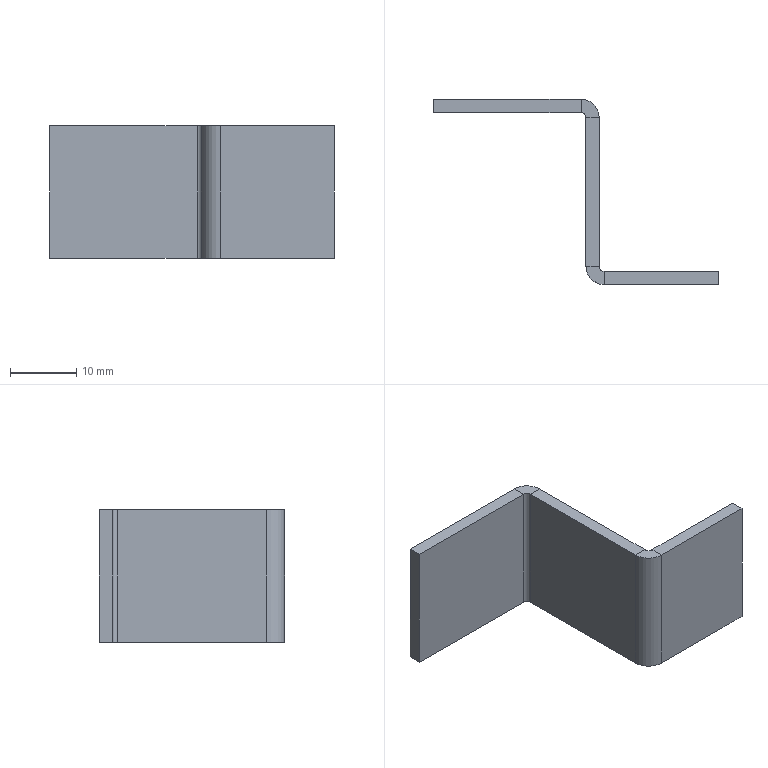Part | SolidWorks | features FlatPattern 1, SMBaseFlange 1, SheetMetal 1 | 1 solid | 22 faces | box 43 x 28 x 20 mm | volume 2700 mm3 | plane 18 | cylinder 4 | commonest cylinder face diameters 1.473 x2 5.473 x2
STEP:
#1=CARTESIAN_POINT('',(25.,-2.737,10.));
#2=VERTEX_POINT('',#1);
#3=CARTESIAN_POINT('',(23.,-2.737,10.));
#4=VERTEX_POINT('',#3);
#5=CARTESIAN_POINT('',(25.,-2.737,10.));
#6=DIRECTION('',(-1.,0.,0.));
#7=VECTOR('',#6,1000.);
#8=LINE('',#5,#7);
#9=EDGE_CURVE('',#2,#4,#8,.T.);
#10=ORIENTED_EDGE('',*,*,#9,.F.);
#11=CARTESIAN_POINT('',(22.263,0.,10.));
#12=VERTEX_POINT('',#11);
#13=CARTESIAN_POINT('',(22.263,-2.737,10.));
#14=DIRECTION('',(0.,0.,-1.));
#15=DIRECTION('',(1.,0.,0.));
#16=AXIS2_PLACEMENT_3D('',#13,#14,#15);
#17=CIRCLE('',#16,2.737);
#18=EDGE_CURVE('',#12,#2,#17,.T.);
#19=ORIENTED_EDGE('',*,*,#18,.F.);
#20=CARTESIAN_POINT('',(22.263,-2.,10.));
#21=VERTEX_POINT('',#20);
#22=CARTESIAN_POINT('',(22.263,-2.,10.));
#23=DIRECTION('',(0.,1.,0.));
#24=VECTOR('',#23,1000.);
#25=LINE('',#22,#24);
#26=EDGE_CURVE('',#21,#12,#25,.T.);
#27=ORIENTED_EDGE('',*,*,#26,.F.);
#28=CARTESIAN_POINT('',(22.263,-2.737,10.));
#29=DIRECTION('',(0.,0.,-1.));
#30=DIRECTION('',(1.,0.,0.));
#31=AXIS2_PLACEMENT_3D('',#28,#29,#30);
#32=CIRCLE('',#31,0.7366);
#33=EDGE_CURVE('',#21,#4,#32,.T.);
#34=ORIENTED_EDGE('',*,*,#33,.T.);
#35=EDGE_LOOP('',(#10,#19,#27,#34));
#36=FACE_OUTER_BOUND('',#35,.T.);
#37=CARTESIAN_POINT('',(25.,-2.737,10.));
#38=DIRECTION('',(0.,0.,1.));
#39=DIRECTION('',(1.,0.,0.));
#40=AXIS2_PLACEMENT_3D('',#37,#38,#39);
#41=PLANE('',#40);
#42=ADVANCED_FACE('',(#36),#41,.T.);
#43=CARTESIAN_POINT('',(25.,-25.263,10.));
#44=VERTEX_POINT('',#43);
#45=CARTESIAN_POINT('',(25.,0.,10.));
#46=DIRECTION('',(0.,-1.,0.));
#47=VECTOR('',#46,1000.);
#48=LINE('',#45,#47);
#49=EDGE_CURVE('',#2,#44,#48,.T.);
#50=ORIENTED_EDGE('',*,*,#49,.F.);
#51=ORIENTED_EDGE('',*,*,#9,.T.);
#52=CARTESIAN_POINT('',(23.,-25.263,10.));
#53=VERTEX_POINT('',#52);
#54=CARTESIAN_POINT('',(23.,0.,10.));
#55=DIRECTION('',(0.,-1.,0.));
#56=VECTOR('',#55,1000.);
#57=LINE('',#54,#56);
#58=EDGE_CURVE('',#4,#53,#57,.T.);
#59=ORIENTED_EDGE('',*,*,#58,.T.);
#60=CARTESIAN_POINT('',(23.,-25.263,10.));
#61=DIRECTION('',(1.,0.,0.));
#62=VECTOR('',#61,1000.);
#63=LINE('',#60,#62);
#64=EDGE_CURVE('',#53,#44,#63,.T.);
#65=ORIENTED_EDGE('',*,*,#64,.T.);
#66=EDGE_LOOP('',(#50,#51,#59,#65));
#67=FACE_OUTER_BOUND('',#66,.T.);
#68=CARTESIAN_POINT('',(22.263,-2.,10.));
#69=DIRECTION('',(0.,0.,1.));
#70=DIRECTION('',(1.,0.,0.));
#71=AXIS2_PLACEMENT_3D('',#68,#69,#70);
#72=PLANE('',#71);
#73=ADVANCED_FACE('',(#67),#72,.T.);
#74=CARTESIAN_POINT('',(22.263,0.,-10.));
#75=VERTEX_POINT('',#74);
#76=CARTESIAN_POINT('',(22.263,-2.,-10.));
#77=VERTEX_POINT('',#76);
#78=CARTESIAN_POINT('',(22.263,0.,-10.));
#79=DIRECTION('',(0.,-1.,0.));
#80=VECTOR('',#79,1000.);
#81=LINE('',#78,#80);
#82=EDGE_CURVE('',#75,#77,#81,.T.);
#83=ORIENTED_EDGE('',*,*,#82,.F.);
#84=CARTESIAN_POINT('',(25.,-2.737,-10.));
#85=VERTEX_POINT('',#84);
#86=CARTESIAN_POINT('',(22.263,-2.737,-10.));
#87=DIRECTION('',(0.,0.,-1.));
#88=DIRECTION('',(1.,0.,0.));
#89=AXIS2_PLACEMENT_3D('',#86,#87,#88);
#90=CIRCLE('',#89,2.737);
#91=EDGE_CURVE('',#75,#85,#90,.T.);
#92=ORIENTED_EDGE('',*,*,#91,.T.);
#93=CARTESIAN_POINT('',(23.,-2.737,-10.));
#94=VERTEX_POINT('',#93);
#95=CARTESIAN_POINT('',(23.,-2.737,-10.));
#96=DIRECTION('',(1.,0.,0.));
#97=VECTOR('',#96,1000.);
#98=LINE('',#95,#97);
#99=EDGE_CURVE('',#94,#85,#98,.T.);
#100=ORIENTED_EDGE('',*,*,#99,.F.);
#101=CARTESIAN_POINT('',(22.263,-2.737,-10.));
#102=DIRECTION('',(0.,0.,-1.));
#103=DIRECTION('',(1.,0.,0.));
#104=AXIS2_PLACEMENT_3D('',#101,#102,#103);
#105=CIRCLE('',#104,0.7366);
#106=EDGE_CURVE('',#77,#94,#105,.T.);
#107=ORIENTED_EDGE('',*,*,#106,.F.);
#108=EDGE_LOOP('',(#83,#92,#100,#107));
#109=FACE_OUTER_BOUND('',#108,.T.);
#110=CARTESIAN_POINT('',(22.263,0.,-10.));
#111=DIRECTION('',(0.,0.,-1.));
#112=DIRECTION('',(-1.,0.,0.));
#113=AXIS2_PLACEMENT_3D('',#110,#111,#112);
#114=PLANE('',#113);
#115=ADVANCED_FACE('',(#109),#114,.T.);
#116=CARTESIAN_POINT('',(0.,0.,-10.));
#117=VERTEX_POINT('',#116);
#118=CARTESIAN_POINT('',(0.,0.,-10.));
#119=DIRECTION('',(1.,0.,0.));
#120=VECTOR('',#119,1000.);
#121=LINE('',#118,#120);
#122=EDGE_CURVE('',#117,#75,#121,.T.);
#123=ORIENTED_EDGE('',*,*,#122,.T.);
#124=ORIENTED_EDGE('',*,*,#82,.T.);
#125=CARTESIAN_POINT('',(0.,-2.,-10.));
#126=VERTEX_POINT('',#125);
#127=CARTESIAN_POINT('',(0.,-2.,-10.));
#128=DIRECTION('',(1.,0.,0.));
#129=VECTOR('',#128,1000.);
#130=LINE('',#127,#129);
#131=EDGE_CURVE('',#126,#77,#130,.T.);
#132=ORIENTED_EDGE('',*,*,#131,.F.);
#133=CARTESIAN_POINT('',(0.,-2.,-10.));
#134=DIRECTION('',(0.,1.,0.));
#135=VECTOR('',#134,1000.);
#136=LINE('',#133,#135);
#137=EDGE_CURVE('',#126,#117,#136,.T.);
#138=ORIENTED_EDGE('',*,*,#137,.T.);
#139=EDGE_LOOP('',(#123,#124,#132,#138));
#140=FACE_OUTER_BOUND('',#139,.T.);
#141=CARTESIAN_POINT('',(23.,-2.737,-10.));
#142=DIRECTION('',(0.,0.,-1.));
#143=DIRECTION('',(-1.,0.,0.));
#144=AXIS2_PLACEMENT_3D('',#141,#142,#143);
#145=PLANE('',#144);
#146=ADVANCED_FACE('',(#140),#145,.T.);
#147=CARTESIAN_POINT('',(25.737,-26.,10.));
#148=VERTEX_POINT('',#147);
#149=CARTESIAN_POINT('',(25.737,-28.,10.));
#150=VERTEX_POINT('',#149);
#151=CARTESIAN_POINT('',(25.737,-26.,10.));
#152=DIRECTION('',(0.,-1.,0.));
#153=VECTOR('',#152,1000.);
#154=LINE('',#151,#153);
#155=EDGE_CURVE('',#148,#150,#154,.T.);
#156=ORIENTED_EDGE('',*,*,#155,.F.);
#157=CARTESIAN_POINT('',(25.737,-25.263,10.));
#158=DIRECTION('',(0.,0.,1.));
#159=DIRECTION('',(-1.,0.,0.));
#160=AXIS2_PLACEMENT_3D('',#157,#158,#159);
#161=CIRCLE('',#160,0.7366);
#162=EDGE_CURVE('',#44,#148,#161,.T.);
#163=ORIENTED_EDGE('',*,*,#162,.F.);
#164=ORIENTED_EDGE('',*,*,#64,.F.);
#165=CARTESIAN_POINT('',(25.737,-25.263,10.));
#166=DIRECTION('',(0.,0.,1.));
#167=DIRECTION('',(1.,0.,0.));
#168=AXIS2_PLACEMENT_3D('',#165,#166,#167);
#169=CIRCLE('',#168,2.737);
#170=EDGE_CURVE('',#53,#150,#169,.T.);
#171=ORIENTED_EDGE('',*,*,#170,.T.);
#172=EDGE_LOOP('',(#156,#163,#164,#171));
#173=FACE_OUTER_BOUND('',#172,.T.);
#174=CARTESIAN_POINT('',(25.737,-26.,10.));
#175=DIRECTION('',(0.,0.,1.));
#176=DIRECTION('',(1.,0.,0.));
#177=AXIS2_PLACEMENT_3D('',#174,#175,#176);
#178=PLANE('',#177);
#179=ADVANCED_FACE('',(#173),#178,.T.);
#180=CARTESIAN_POINT('',(43.,-26.,10.));
#181=VERTEX_POINT('',#180);
#182=CARTESIAN_POINT('',(25.,-26.,10.));
#183=DIRECTION('',(1.,0.,0.));
#184=VECTOR('',#183,1000.);
#185=LINE('',#182,#184);
#186=EDGE_CURVE('',#148,#181,#185,.T.);
#187=ORIENTED_EDGE('',*,*,#186,.F.);
#188=ORIENTED_EDGE('',*,*,#155,.T.);
#189=CARTESIAN_POINT('',(43.,-28.,10.));
#190=VERTEX_POINT('',#189);
#191=CARTESIAN_POINT('',(25.,-28.,10.));
#192=DIRECTION('',(1.,0.,0.));
#193=VECTOR('',#192,1000.);
#194=LINE('',#191,#193);
#195=EDGE_CURVE('',#150,#190,#194,.T.);
#196=ORIENTED_EDGE('',*,*,#195,.T.);
#197=CARTESIAN_POINT('',(43.,-26.,10.));
#198=DIRECTION('',(0.,-1.,0.));
#199=VECTOR('',#198,1000.);
#200=LINE('',#197,#199);
#201=EDGE_CURVE('',#181,#190,#200,.T.);
#202=ORIENTED_EDGE('',*,*,#201,.F.);
#203=EDGE_LOOP('',(#187,#188,#196,#202));
#204=FACE_OUTER_BOUND('',#203,.T.);
#205=CARTESIAN_POINT('',(23.,-25.263,10.));
#206=DIRECTION('',(0.,0.,1.));
#207=DIRECTION('',(1.,0.,0.));
#208=AXIS2_PLACEMENT_3D('',#205,#206,#207);
#209=PLANE('',#208);
#210=ADVANCED_FACE('',(#204),#209,.T.);
#211=CARTESIAN_POINT('',(25.,-25.263,-10.));
#212=VERTEX_POINT('',#211);
#213=CARTESIAN_POINT('',(23.,-25.263,-10.));
#214=VERTEX_POINT('',#213);
#215=CARTESIAN_POINT('',(25.,-25.263,-10.));
#216=DIRECTION('',(-1.,0.,0.));
#217=VECTOR('',#216,1000.);
#218=LINE('',#215,#217);
#219=EDGE_CURVE('',#212,#214,#218,.T.);
#220=ORIENTED_EDGE('',*,*,#219,.F.);
#221=CARTESIAN_POINT('',(25.737,-26.,-10.));
#222=VERTEX_POINT('',#221);
#223=CARTESIAN_POINT('',(25.737,-25.263,-10.));
#224=DIRECTION('',(0.,0.,1.));
#225=DIRECTION('',(-1.,0.,0.));
#226=AXIS2_PLACEMENT_3D('',#223,#224,#225);
#227=CIRCLE('',#226,0.7366);
#228=EDGE_CURVE('',#212,#222,#227,.T.);
#229=ORIENTED_EDGE('',*,*,#228,.T.);
#230=CARTESIAN_POINT('',(25.737,-28.,-10.));
#231=VERTEX_POINT('',#230);
#232=CARTESIAN_POINT('',(25.737,-28.,-10.));
#233=DIRECTION('',(0.,1.,0.));
#234=VECTOR('',#233,1000.);
#235=LINE('',#232,#234);
#236=EDGE_CURVE('',#231,#222,#235,.T.);
#237=ORIENTED_EDGE('',*,*,#236,.F.);
#238=CARTESIAN_POINT('',(25.737,-25.263,-10.));
#239=DIRECTION('',(0.,0.,1.));
#240=DIRECTION('',(1.,0.,0.));
#241=AXIS2_PLACEMENT_3D('',#238,#239,#240);
#242=CIRCLE('',#241,2.737);
#243=EDGE_CURVE('',#214,#231,#242,.T.);
#244=ORIENTED_EDGE('',*,*,#243,.F.);
#245=EDGE_LOOP('',(#220,#229,#237,#244));
#246=FACE_OUTER_BOUND('',#245,.T.);
#247=CARTESIAN_POINT('',(25.,-25.263,-10.));
#248=DIRECTION('',(0.,0.,-1.));
#249=DIRECTION('',(-1.,0.,0.));
#250=AXIS2_PLACEMENT_3D('',#247,#248,#249);
#251=PLANE('',#250);
#252=ADVANCED_FACE('',(#246),#251,.T.);
#253=CARTESIAN_POINT('',(25.,0.,-10.));
#254=DIRECTION('',(0.,-1.,0.));
#255=VECTOR('',#254,1000.);
#256=LINE('',#253,#255);
#257=EDGE_CURVE('',#85,#212,#256,.T.);
#258=ORIENTED_EDGE('',*,*,#257,.T.);
#259=ORIENTED_EDGE('',*,*,#219,.T.);
#260=CARTESIAN_POINT('',(23.,0.,-10.));
#261=DIRECTION('',(0.,-1.,0.));
#262=VECTOR('',#261,1000.);
#263=LINE('',#260,#262);
#264=EDGE_CURVE('',#94,#214,#263,.T.);
#265=ORIENTED_EDGE('',*,*,#264,.F.);
#266=ORIENTED_EDGE('',*,*,#99,.T.);
#267=EDGE_LOOP('',(#258,#259,#265,#266));
#268=FACE_OUTER_BOUND('',#267,.T.);
#269=CARTESIAN_POINT('',(25.737,-28.,-10.));
#270=DIRECTION('',(0.,0.,-1.));
#271=DIRECTION('',(-1.,0.,0.));
#272=AXIS2_PLACEMENT_3D('',#269,#270,#271);
#273=PLANE('',#272);
#274=ADVANCED_FACE('',(#268),#273,.T.);
#275=CARTESIAN_POINT('',(43.,-28.,-10.));
#276=VERTEX_POINT('',#275);
#277=CARTESIAN_POINT('',(25.,-28.,-10.));
#278=DIRECTION('',(1.,0.,0.));
#279=VECTOR('',#278,1000.);
#280=LINE('',#277,#279);
#281=EDGE_CURVE('',#231,#276,#280,.T.);
#282=ORIENTED_EDGE('',*,*,#281,.T.);
#283=CARTESIAN_POINT('',(43.,-28.,10.));
#284=DIRECTION('',(0.,0.,-1.));
#285=VECTOR('',#284,1000.);
#286=LINE('',#283,#285);
#287=EDGE_CURVE('',#190,#276,#286,.T.);
#288=ORIENTED_EDGE('',*,*,#287,.F.);
#289=ORIENTED_EDGE('',*,*,#195,.F.);
#290=CARTESIAN_POINT('',(25.737,-28.,10.));
#291=DIRECTION('',(0.,0.,-1.));
#292=VECTOR('',#291,1000.);
#293=LINE('',#290,#292);
#294=EDGE_CURVE('',#150,#231,#293,.T.);
#295=ORIENTED_EDGE('',*,*,#294,.T.);
#296=EDGE_LOOP('',(#282,#288,#289,#295));
#297=FACE_OUTER_BOUND('',#296,.T.);
#298=CARTESIAN_POINT('',(25.,-28.,10.));
#299=DIRECTION('',(0.,1.,0.));
#300=DIRECTION('',(0.,0.,1.));
#301=AXIS2_PLACEMENT_3D('',#298,#299,#300);
#302=PLANE('',#301);
#303=ADVANCED_FACE('',(#297),#302,.F.);
#304=CARTESIAN_POINT('',(43.,-26.,-10.));
#305=VERTEX_POINT('',#304);
#306=CARTESIAN_POINT('',(43.,-26.,-10.));
#307=DIRECTION('',(0.,-1.,0.));
#308=VECTOR('',#307,1000.);
#309=LINE('',#306,#308);
#310=EDGE_CURVE('',#305,#276,#309,.T.);
#311=ORIENTED_EDGE('',*,*,#310,.F.);
#312=CARTESIAN_POINT('',(43.,-26.,10.));
#313=DIRECTION('',(0.,0.,-1.));
#314=VECTOR('',#313,1000.);
#315=LINE('',#312,#314);
#316=EDGE_CURVE('',#181,#305,#315,.T.);
#317=ORIENTED_EDGE('',*,*,#316,.F.);
#318=ORIENTED_EDGE('',*,*,#201,.T.);
#319=ORIENTED_EDGE('',*,*,#287,.T.);
#320=EDGE_LOOP('',(#311,#317,#318,#319));
#321=FACE_OUTER_BOUND('',#320,.T.);
#322=CARTESIAN_POINT('',(43.,-26.,10.));
#323=DIRECTION('',(1.,0.,0.));
#324=DIRECTION('',(0.,0.,-1.));
#325=AXIS2_PLACEMENT_3D('',#322,#323,#324);
#326=PLANE('',#325);
#327=ADVANCED_FACE('',(#321),#326,.T.);
#328=CARTESIAN_POINT('',(25.,-26.,-10.));
#329=DIRECTION('',(1.,0.,0.));
#330=VECTOR('',#329,1000.);
#331=LINE('',#328,#330);
#332=EDGE_CURVE('',#222,#305,#331,.T.);
#333=ORIENTED_EDGE('',*,*,#332,.F.);
#334=CARTESIAN_POINT('',(25.737,-26.,10.));
#335=DIRECTION('',(0.,0.,-1.));
#336=VECTOR('',#335,1000.);
#337=LINE('',#334,#336);
#338=EDGE_CURVE('',#148,#222,#337,.T.);
#339=ORIENTED_EDGE('',*,*,#338,.F.);
#340=ORIENTED_EDGE('',*,*,#186,.T.);
#341=ORIENTED_EDGE('',*,*,#316,.T.);
#342=EDGE_LOOP('',(#333,#339,#340,#341));
#343=FACE_OUTER_BOUND('',#342,.T.);
#344=CARTESIAN_POINT('',(25.,-26.,10.));
#345=DIRECTION('',(0.,1.,0.));
#346=DIRECTION('',(0.,0.,1.));
#347=AXIS2_PLACEMENT_3D('',#344,#345,#346);
#348=PLANE('',#347);
#349=ADVANCED_FACE('',(#343),#348,.T.);
#350=ORIENTED_EDGE('',*,*,#228,.F.);
#351=CARTESIAN_POINT('',(25.,-25.263,10.));
#352=DIRECTION('',(0.,0.,-1.));
#353=VECTOR('',#352,1000.);
#354=LINE('',#351,#353);
#355=EDGE_CURVE('',#44,#212,#354,.T.);
#356=ORIENTED_EDGE('',*,*,#355,.F.);
#357=ORIENTED_EDGE('',*,*,#162,.T.);
#358=ORIENTED_EDGE('',*,*,#338,.T.);
#359=EDGE_LOOP('',(#350,#356,#357,#358));
#360=FACE_OUTER_BOUND('',#359,.T.);
#361=CARTESIAN_POINT('',(25.737,-25.263,10.));
#362=DIRECTION('',(0.,0.,-1.));
#363=DIRECTION('',(-1.,0.,0.));
#364=AXIS2_PLACEMENT_3D('',#361,#362,#363);
#365=CYLINDRICAL_SURFACE('',#364,0.7366);
#366=ADVANCED_FACE('',(#360),#365,.F.);
#367=ORIENTED_EDGE('',*,*,#257,.F.);
#368=CARTESIAN_POINT('',(25.,-2.737,10.));
#369=DIRECTION('',(0.,0.,-1.));
#370=VECTOR('',#369,1000.);
#371=LINE('',#368,#370);
#372=EDGE_CURVE('',#2,#85,#371,.T.);
#373=ORIENTED_EDGE('',*,*,#372,.F.);
#374=ORIENTED_EDGE('',*,*,#49,.T.);
#375=ORIENTED_EDGE('',*,*,#355,.T.);
#376=EDGE_LOOP('',(#367,#373,#374,#375));
#377=FACE_OUTER_BOUND('',#376,.T.);
#378=CARTESIAN_POINT('',(25.,0.,10.));
#379=DIRECTION('',(1.,0.,0.));
#380=DIRECTION('',(0.,0.,-1.));
#381=AXIS2_PLACEMENT_3D('',#378,#379,#380);
#382=PLANE('',#381);
#383=ADVANCED_FACE('',(#377),#382,.T.);
#384=ORIENTED_EDGE('',*,*,#91,.F.);
#385=CARTESIAN_POINT('',(22.263,0.,10.));
#386=DIRECTION('',(0.,0.,-1.));
#387=VECTOR('',#386,1000.);
#388=LINE('',#385,#387);
#389=EDGE_CURVE('',#12,#75,#388,.T.);
#390=ORIENTED_EDGE('',*,*,#389,.F.);
#391=ORIENTED_EDGE('',*,*,#18,.T.);
#392=ORIENTED_EDGE('',*,*,#372,.T.);
#393=EDGE_LOOP('',(#384,#390,#391,#392));
#394=FACE_OUTER_BOUND('',#393,.T.);
#395=CARTESIAN_POINT('',(22.263,-2.737,10.));
#396=DIRECTION('',(0.,0.,-1.));
#397=DIRECTION('',(-1.,0.,0.));
#398=AXIS2_PLACEMENT_3D('',#395,#396,#397);
#399=CYLINDRICAL_SURFACE('',#398,2.737);
#400=ADVANCED_FACE('',(#394),#399,.T.);
#401=ORIENTED_EDGE('',*,*,#122,.F.);
#402=CARTESIAN_POINT('',(0.,0.,10.));
#403=VERTEX_POINT('',#402);
#404=CARTESIAN_POINT('',(0.,0.,10.));
#405=DIRECTION('',(0.,0.,-1.));
#406=VECTOR('',#405,1000.);
#407=LINE('',#404,#406);
#408=EDGE_CURVE('',#403,#117,#407,.T.);
#409=ORIENTED_EDGE('',*,*,#408,.F.);
#410=CARTESIAN_POINT('',(0.,0.,10.));
#411=DIRECTION('',(1.,0.,0.));
#412=VECTOR('',#411,1000.);
#413=LINE('',#410,#412);
#414=EDGE_CURVE('',#403,#12,#413,.T.);
#415=ORIENTED_EDGE('',*,*,#414,.T.);
#416=ORIENTED_EDGE('',*,*,#389,.T.);
#417=EDGE_LOOP('',(#401,#409,#415,#416));
#418=FACE_OUTER_BOUND('',#417,.T.);
#419=CARTESIAN_POINT('',(0.,0.,10.));
#420=DIRECTION('',(0.,1.,0.));
#421=DIRECTION('',(0.,0.,1.));
#422=AXIS2_PLACEMENT_3D('',#419,#420,#421);
#423=PLANE('',#422);
#424=ADVANCED_FACE('',(#418),#423,.T.);
#425=ORIENTED_EDGE('',*,*,#137,.F.);
#426=CARTESIAN_POINT('',(0.,-2.,10.));
#427=VERTEX_POINT('',#426);
#428=CARTESIAN_POINT('',(0.,-2.,10.));
#429=DIRECTION('',(0.,0.,-1.));
#430=VECTOR('',#429,1000.);
#431=LINE('',#428,#430);
#432=EDGE_CURVE('',#427,#126,#431,.T.);
#433=ORIENTED_EDGE('',*,*,#432,.F.);
#434=CARTESIAN_POINT('',(0.,-2.,10.));
#435=DIRECTION('',(0.,1.,0.));
#436=VECTOR('',#435,1000.);
#437=LINE('',#434,#436);
#438=EDGE_CURVE('',#427,#403,#437,.T.);
#439=ORIENTED_EDGE('',*,*,#438,.T.);
#440=ORIENTED_EDGE('',*,*,#408,.T.);
#441=EDGE_LOOP('',(#425,#433,#439,#440));
#442=FACE_OUTER_BOUND('',#441,.T.);
#443=CARTESIAN_POINT('',(0.,-2.,10.));
#444=DIRECTION('',(-1.,0.,0.));
#445=DIRECTION('',(0.,0.,1.));
#446=AXIS2_PLACEMENT_3D('',#443,#444,#445);
#447=PLANE('',#446);
#448=ADVANCED_FACE('',(#442),#447,.T.);
#449=ORIENTED_EDGE('',*,*,#131,.T.);
#450=CARTESIAN_POINT('',(22.263,-2.,10.));
#451=DIRECTION('',(0.,0.,-1.));
#452=VECTOR('',#451,1000.);
#453=LINE('',#450,#452);
#454=EDGE_CURVE('',#21,#77,#453,.T.);
#455=ORIENTED_EDGE('',*,*,#454,.F.);
#456=CARTESIAN_POINT('',(0.,-2.,10.));
#457=DIRECTION('',(1.,0.,0.));
#458=VECTOR('',#457,1000.);
#459=LINE('',#456,#458);
#460=EDGE_CURVE('',#427,#21,#459,.T.);
#461=ORIENTED_EDGE('',*,*,#460,.F.);
#462=ORIENTED_EDGE('',*,*,#432,.T.);
#463=EDGE_LOOP('',(#449,#455,#461,#462));
#464=FACE_OUTER_BOUND('',#463,.T.);
#465=CARTESIAN_POINT('',(0.,-2.,10.));
#466=DIRECTION('',(0.,1.,0.));
#467=DIRECTION('',(0.,0.,1.));
#468=AXIS2_PLACEMENT_3D('',#465,#466,#467);
#469=PLANE('',#468);
#470=ADVANCED_FACE('',(#464),#469,.F.);
#471=ORIENTED_EDGE('',*,*,#106,.T.);
#472=CARTESIAN_POINT('',(23.,-2.737,10.));
#473=DIRECTION('',(0.,0.,-1.));
#474=VECTOR('',#473,1000.);
#475=LINE('',#472,#474);
#476=EDGE_CURVE('',#4,#94,#475,.T.);
#477=ORIENTED_EDGE('',*,*,#476,.F.);
#478=ORIENTED_EDGE('',*,*,#33,.F.);
#479=ORIENTED_EDGE('',*,*,#454,.T.);
#480=EDGE_LOOP('',(#471,#477,#478,#479));
#481=FACE_OUTER_BOUND('',#480,.T.);
#482=CARTESIAN_POINT('',(22.263,-2.737,10.));
#483=DIRECTION('',(0.,0.,-1.));
#484=DIRECTION('',(-1.,0.,0.));
#485=AXIS2_PLACEMENT_3D('',#482,#483,#484);
#486=CYLINDRICAL_SURFACE('',#485,0.7366);
#487=ADVANCED_FACE('',(#481),#486,.F.);
#488=ORIENTED_EDGE('',*,*,#264,.T.);
#489=CARTESIAN_POINT('',(23.,-25.263,10.));
#490=DIRECTION('',(0.,0.,-1.));
#491=VECTOR('',#490,1000.);
#492=LINE('',#489,#491);
#493=EDGE_CURVE('',#53,#214,#492,.T.);
#494=ORIENTED_EDGE('',*,*,#493,.F.);
#495=ORIENTED_EDGE('',*,*,#58,.F.);
#496=ORIENTED_EDGE('',*,*,#476,.T.);
#497=EDGE_LOOP('',(#488,#494,#495,#496));
#498=FACE_OUTER_BOUND('',#497,.T.);
#499=CARTESIAN_POINT('',(23.,0.,10.));
#500=DIRECTION('',(1.,0.,0.));
#501=DIRECTION('',(0.,0.,-1.));
#502=AXIS2_PLACEMENT_3D('',#499,#500,#501);
#503=PLANE('',#502);
#504=ADVANCED_FACE('',(#498),#503,.F.);
#505=ORIENTED_EDGE('',*,*,#243,.T.);
#506=ORIENTED_EDGE('',*,*,#294,.F.);
#507=ORIENTED_EDGE('',*,*,#170,.F.);
#508=ORIENTED_EDGE('',*,*,#493,.T.);
#509=EDGE_LOOP('',(#505,#506,#507,#508));
#510=FACE_OUTER_BOUND('',#509,.T.);
#511=CARTESIAN_POINT('',(25.737,-25.263,10.));
#512=DIRECTION('',(0.,0.,-1.));
#513=DIRECTION('',(-1.,0.,0.));
#514=AXIS2_PLACEMENT_3D('',#511,#512,#513);
#515=CYLINDRICAL_SURFACE('',#514,2.737);
#516=ADVANCED_FACE('',(#510),#515,.T.);
#517=ORIENTED_EDGE('',*,*,#460,.T.);
#518=ORIENTED_EDGE('',*,*,#26,.T.);
#519=ORIENTED_EDGE('',*,*,#414,.F.);
#520=ORIENTED_EDGE('',*,*,#438,.F.);
#521=EDGE_LOOP('',(#517,#518,#519,#520));
#522=FACE_OUTER_BOUND('',#521,.T.);
#523=CARTESIAN_POINT('',(25.737,-25.263,10.));
#524=DIRECTION('',(0.,0.,-1.));
#525=DIRECTION('',(-1.,0.,0.));
#526=AXIS2_PLACEMENT_3D('',#523,#524,#525);
#527=PLANE('',#526);
#528=ADVANCED_FACE('',(#522),#527,.F.);
#529=ORIENTED_EDGE('',*,*,#281,.F.);
#530=ORIENTED_EDGE('',*,*,#236,.T.);
#531=ORIENTED_EDGE('',*,*,#332,.T.);
#532=ORIENTED_EDGE('',*,*,#310,.T.);
#533=EDGE_LOOP('',(#529,#530,#531,#532));
#534=FACE_OUTER_BOUND('',#533,.T.);
#535=CARTESIAN_POINT('',(25.737,-25.263,-10.));
#536=DIRECTION('',(0.,0.,-1.));
#537=DIRECTION('',(-1.,0.,0.));
#538=AXIS2_PLACEMENT_3D('',#535,#536,#537);
#539=PLANE('',#538);
#540=ADVANCED_FACE('',(#534),#539,.T.);
#541=CLOSED_SHELL('',(#42,#73,#115,#146,#179,#210,#252,#274,#303,#327,#349,#366,#383,#400,#424,#448,#470,#487,#504,#516,#528,#540));
#542=MANIFOLD_SOLID_BREP('',#541);
#543=CARTESIAN_POINT('',(0.,0.,0.));
#544=DIRECTION('',(0.,0.,1.));
#545=DIRECTION('',(1.,0.,0.));
#546=AXIS2_PLACEMENT_3D('',#543,#544,#545);
#547=(LENGTH_UNIT()NAMED_UNIT(*)SI_UNIT(.MILLI.,.METRE.));
#548=UNCERTAINTY_MEASURE_WITH_UNIT(LENGTH_MEASURE(0.00001),#547,'','');
#549=(NAMED_UNIT(*)PLANE_ANGLE_UNIT()SI_UNIT($,.RADIAN.));
#550=(NAMED_UNIT(*)SI_UNIT($,.STERADIAN.)SOLID_ANGLE_UNIT());
#551=(GEOMETRIC_REPRESENTATION_CONTEXT(3)GLOBAL_UNCERTAINTY_ASSIGNED_CONTEXT((#548))GLOBAL_UNIT_ASSIGNED_CONTEXT((#547,#549,#550))REPRESENTATION_CONTEXT('',''));
#552=ADVANCED_BREP_SHAPE_REPRESENTATION('',(#542,#546),#551);